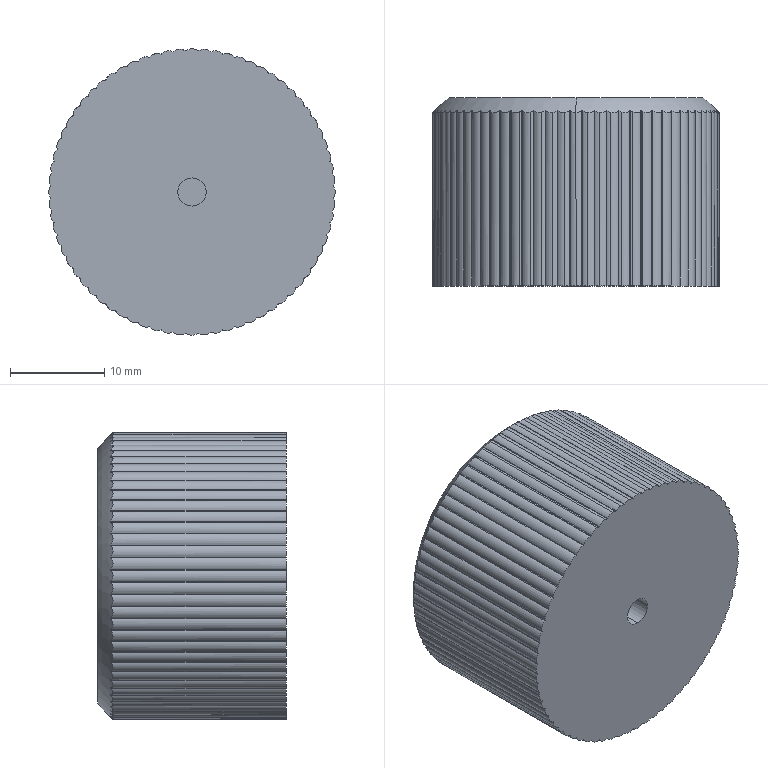Part | STEP file | PLASMA_KNOB_SIZE | 1 solid | 166 faces | box 30.4 x 20 x 30.4 mm | volume 14168 mm3 | cylinder 161 | plane 3 | torus 2 | commonest cylinder face diameters 2 x87 30 x72 3 x2